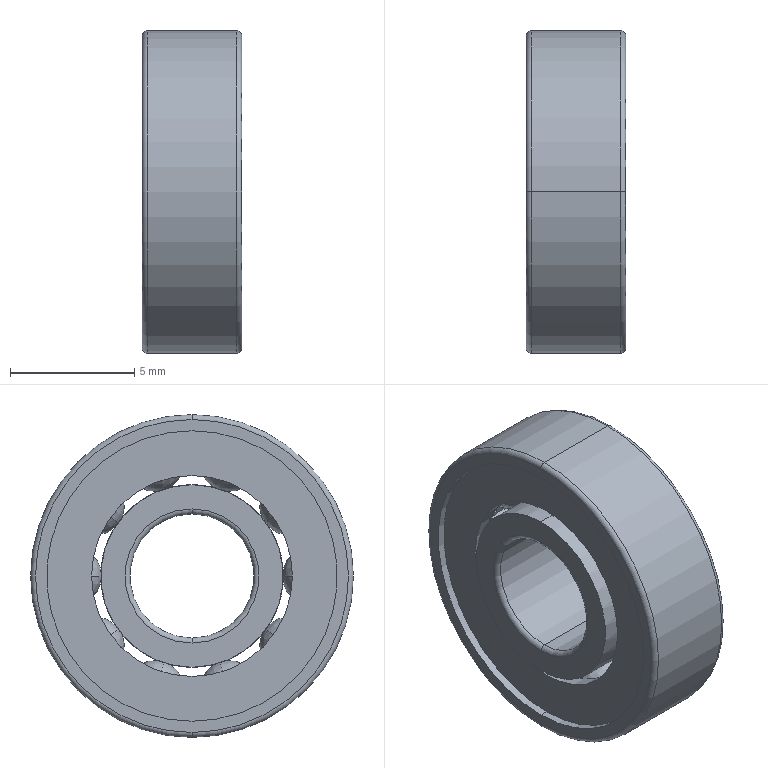Part | NX | features BREP 1 | 1 solid | 173 faces | box 4 x 13 x 13 mm | volume 316.169 mm3 | sphere 80 | torus 41 | plane 28 | cylinder 24 | commonest cylinder face diameters 11.7 x8 7.35 x4 8.096 x4 5 x2 8.903 x2 10.146 x2